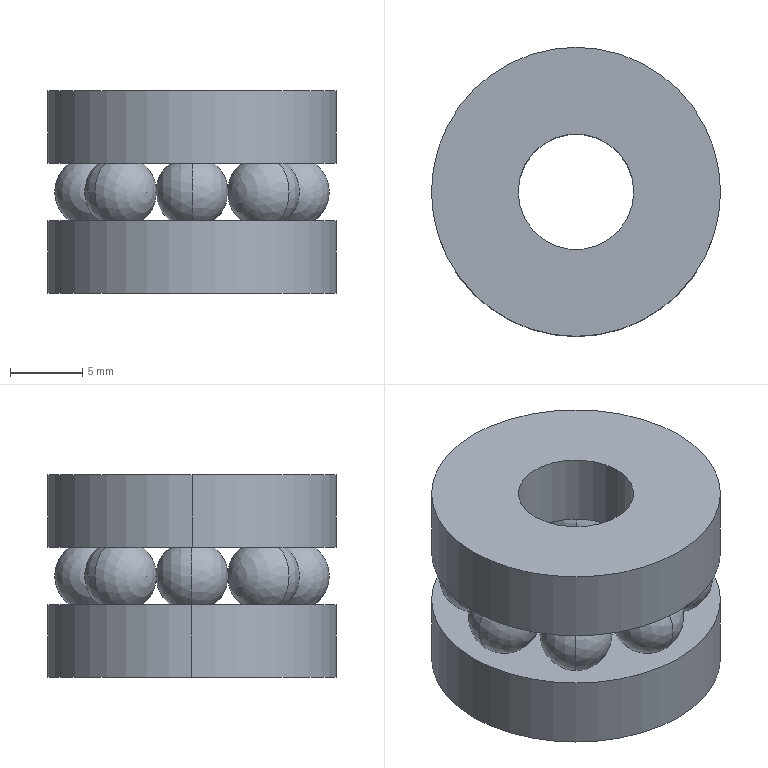Part | SolidWorks | features CirPattern 1, Extrusion 1, ICE 1, Revolution 1 | 1 solid | 28 faces | box 20 x 20 x 14 mm | volume 3133 mm3 | sphere 16 | cylinder 8 | plane 4 | commonest cylinder face diameters 8 x4 20 x4
STEP:
#1=CARTESIAN_POINT('',(-4.,0.,-4.));
#2=VERTEX_POINT('',#1);
#3=CARTESIAN_POINT('',(4.,0.,-4.));
#4=VERTEX_POINT('',#3);
#5=CARTESIAN_POINT('',(0.,0.,-4.));
#6=DIRECTION('',(0.,0.,1.));
#7=DIRECTION('',(1.,0.,0.));
#8=AXIS2_PLACEMENT_3D('',#5,#6,#7);
#9=CIRCLE('',#8,4.);
#10=EDGE_CURVE('',#2,#4,#9,.T.);
#11=ORIENTED_EDGE('',*,*,#10,.F.);
#12=CARTESIAN_POINT('',(-4.,0.,1.));
#13=VERTEX_POINT('',#12);
#14=CARTESIAN_POINT('',(-4.,0.,-4.));
#15=DIRECTION('',(0.,0.,1.));
#16=VECTOR('',#15,1000.);
#17=LINE('',#14,#16);
#18=EDGE_CURVE('',#2,#13,#17,.T.);
#19=ORIENTED_EDGE('',*,*,#18,.T.);
#20=CARTESIAN_POINT('',(4.,0.,1.));
#21=VERTEX_POINT('',#20);
#22=CARTESIAN_POINT('',(0.,0.,1.));
#23=DIRECTION('',(0.,0.,1.));
#24=DIRECTION('',(1.,0.,0.));
#25=AXIS2_PLACEMENT_3D('',#22,#23,#24);
#26=CIRCLE('',#25,4.);
#27=EDGE_CURVE('',#13,#21,#26,.T.);
#28=ORIENTED_EDGE('',*,*,#27,.T.);
#29=CARTESIAN_POINT('',(4.,0.,-4.));
#30=DIRECTION('',(0.,0.,1.));
#31=VECTOR('',#30,1000.);
#32=LINE('',#29,#31);
#33=EDGE_CURVE('',#4,#21,#32,.T.);
#34=ORIENTED_EDGE('',*,*,#33,.F.);
#35=EDGE_LOOP('',(#11,#19,#28,#34));
#36=FACE_OUTER_BOUND('',#35,.T.);
#37=CARTESIAN_POINT('',(0.,0.,-4.));
#38=DIRECTION('',(0.,0.,1.));
#39=DIRECTION('',(1.,0.,0.));
#40=AXIS2_PLACEMENT_3D('',#37,#38,#39);
#41=CYLINDRICAL_SURFACE('',#40,4.);
#42=ADVANCED_FACE('',(#36),#41,.F.);
#43=CARTESIAN_POINT('',(10.,0.,-4.));
#44=VERTEX_POINT('',#43);
#45=CARTESIAN_POINT('',(-10.,0.,-4.));
#46=VERTEX_POINT('',#45);
#47=CARTESIAN_POINT('',(0.,0.,-4.));
#48=DIRECTION('',(0.,0.,1.));
#49=DIRECTION('',(1.,0.,0.));
#50=AXIS2_PLACEMENT_3D('',#47,#48,#49);
#51=CIRCLE('',#50,10.);
#52=EDGE_CURVE('',#44,#46,#51,.T.);
#53=ORIENTED_EDGE('',*,*,#52,.T.);
#54=CARTESIAN_POINT('',(-10.,0.,1.));
#55=VERTEX_POINT('',#54);
#56=CARTESIAN_POINT('',(-10.,0.,-4.));
#57=DIRECTION('',(0.,0.,1.));
#58=VECTOR('',#57,1000.);
#59=LINE('',#56,#58);
#60=EDGE_CURVE('',#46,#55,#59,.T.);
#61=ORIENTED_EDGE('',*,*,#60,.T.);
#62=CARTESIAN_POINT('',(10.,0.,1.));
#63=VERTEX_POINT('',#62);
#64=CARTESIAN_POINT('',(0.,0.,1.));
#65=DIRECTION('',(0.,0.,1.));
#66=DIRECTION('',(1.,0.,0.));
#67=AXIS2_PLACEMENT_3D('',#64,#65,#66);
#68=CIRCLE('',#67,10.);
#69=EDGE_CURVE('',#63,#55,#68,.T.);
#70=ORIENTED_EDGE('',*,*,#69,.F.);
#71=CARTESIAN_POINT('',(10.,0.,-4.));
#72=DIRECTION('',(0.,0.,1.));
#73=VECTOR('',#72,1000.);
#74=LINE('',#71,#73);
#75=EDGE_CURVE('',#44,#63,#74,.T.);
#76=ORIENTED_EDGE('',*,*,#75,.F.);
#77=EDGE_LOOP('',(#53,#61,#70,#76));
#78=FACE_OUTER_BOUND('',#77,.T.);
#79=CARTESIAN_POINT('',(0.,0.,-4.));
#80=DIRECTION('',(0.,0.,1.));
#81=DIRECTION('',(1.,0.,0.));
#82=AXIS2_PLACEMENT_3D('',#79,#80,#81);
#83=CYLINDRICAL_SURFACE('',#82,10.);
#84=ADVANCED_FACE('',(#78),#83,.T.);
#85=CARTESIAN_POINT('',(-6.718,6.718,3.));
#86=VERTEX_POINT('',#85);
#87=CARTESIAN_POINT('',(-6.01,6.01,5.));
#88=VERTEX_POINT('',#87);
#89=CARTESIAN_POINT('',(-4.95,4.95,3.));
#90=DIRECTION('',(0.7071,0.7071,0.));
#91=DIRECTION('',(-0.7071,0.7071,0.));
#92=AXIS2_PLACEMENT_3D('',#89,#90,#91);
#93=CIRCLE('',#92,2.5);
#94=EDGE_CURVE('',#86,#88,#93,.T.);
#95=ORIENTED_EDGE('',*,*,#94,.F.);
#96=CARTESIAN_POINT('',(-6.01,6.01,1.));
#97=VERTEX_POINT('',#96);
#98=CARTESIAN_POINT('',(-4.95,4.95,3.));
#99=DIRECTION('',(-0.7071,-0.7071,0.));
#100=DIRECTION('',(0.7071,-0.7071,0.));
#101=AXIS2_PLACEMENT_3D('',#98,#99,#100);
#102=CIRCLE('',#101,2.5);
#103=EDGE_CURVE('',#86,#97,#102,.T.);
#104=ORIENTED_EDGE('',*,*,#103,.T.);
#105=CARTESIAN_POINT('',(-3.889,3.889,1.));
#106=VERTEX_POINT('',#105);
#107=CARTESIAN_POINT('',(-4.95,4.95,1.));
#108=DIRECTION('',(0.,0.,1.));
#109=DIRECTION('',(1.,0.,0.));
#110=AXIS2_PLACEMENT_3D('',#107,#108,#109);
#111=CIRCLE('',#110,1.5);
#112=EDGE_CURVE('',#97,#106,#111,.T.);
#113=ORIENTED_EDGE('',*,*,#112,.T.);
#114=CARTESIAN_POINT('',(-3.182,3.182,3.));
#115=VERTEX_POINT('',#114);
#116=CARTESIAN_POINT('',(-4.95,4.95,3.));
#117=DIRECTION('',(-0.7071,-0.7071,0.));
#118=DIRECTION('',(0.7071,-0.7071,0.));
#119=AXIS2_PLACEMENT_3D('',#116,#117,#118);
#120=CIRCLE('',#119,2.5);
#121=EDGE_CURVE('',#106,#115,#120,.T.);
#122=ORIENTED_EDGE('',*,*,#121,.T.);
#123=CARTESIAN_POINT('',(-3.889,3.889,5.));
#124=VERTEX_POINT('',#123);
#125=CARTESIAN_POINT('',(-4.95,4.95,3.));
#126=DIRECTION('',(0.7071,0.7071,0.));
#127=DIRECTION('',(-0.7071,0.7071,0.));
#128=AXIS2_PLACEMENT_3D('',#125,#126,#127);
#129=CIRCLE('',#128,2.5);
#130=EDGE_CURVE('',#124,#115,#129,.T.);
#131=ORIENTED_EDGE('',*,*,#130,.F.);
#132=CARTESIAN_POINT('',(-4.95,4.95,5.));
#133=DIRECTION('',(0.,0.,-1.));
#134=DIRECTION('',(1.,0.,0.));
#135=AXIS2_PLACEMENT_3D('',#132,#133,#134);
#136=CIRCLE('',#135,1.5);
#137=EDGE_CURVE('',#124,#88,#136,.T.);
#138=ORIENTED_EDGE('',*,*,#137,.T.);
#139=EDGE_LOOP('',(#95,#104,#113,#122,#131,#138));
#140=FACE_OUTER_BOUND('',#139,.T.);
#141=CARTESIAN_POINT('',(-4.95,4.95,3.));
#142=DIRECTION('',(-0.7071,-0.7071,0.));
#143=DIRECTION('',(0.,0.,1.));
#144=AXIS2_PLACEMENT_3D('',#141,#142,#143);
#145=SPHERICAL_SURFACE('',#144,2.5);
#146=ADVANCED_FACE('',(#140),#145,.T.);
#147=CARTESIAN_POINT('',(-9.5,0.,3.));
#148=VERTEX_POINT('',#147);
#149=CARTESIAN_POINT('',(-8.5,0.,5.));
#150=VERTEX_POINT('',#149);
#151=CARTESIAN_POINT('',(-7.,0.,3.));
#152=DIRECTION('',(0.,1.,0.));
#153=DIRECTION('',(-1.,0.,0.));
#154=AXIS2_PLACEMENT_3D('',#151,#152,#153);
#155=CIRCLE('',#154,2.5);
#156=EDGE_CURVE('',#148,#150,#155,.T.);
#157=ORIENTED_EDGE('',*,*,#156,.F.);
#158=CARTESIAN_POINT('',(-8.5,0.,1.));
#159=VERTEX_POINT('',#158);
#160=CARTESIAN_POINT('',(-7.,0.,3.));
#161=DIRECTION('',(0.,-1.,0.));
#162=DIRECTION('',(1.,0.,0.));
#163=AXIS2_PLACEMENT_3D('',#160,#161,#162);
#164=CIRCLE('',#163,2.5);
#165=EDGE_CURVE('',#148,#159,#164,.T.);
#166=ORIENTED_EDGE('',*,*,#165,.T.);
#167=CARTESIAN_POINT('',(-5.5,0.,1.));
#168=VERTEX_POINT('',#167);
#169=CARTESIAN_POINT('',(-7.,0.,1.));
#170=DIRECTION('',(0.,0.,1.));
#171=DIRECTION('',(1.,0.,0.));
#172=AXIS2_PLACEMENT_3D('',#169,#170,#171);
#173=CIRCLE('',#172,1.5);
#174=EDGE_CURVE('',#159,#168,#173,.T.);
#175=ORIENTED_EDGE('',*,*,#174,.T.);
#176=CARTESIAN_POINT('',(-4.5,0.,3.));
#177=VERTEX_POINT('',#176);
#178=CARTESIAN_POINT('',(-7.,0.,3.));
#179=DIRECTION('',(0.,-1.,0.));
#180=DIRECTION('',(1.,0.,0.));
#181=AXIS2_PLACEMENT_3D('',#178,#179,#180);
#182=CIRCLE('',#181,2.5);
#183=EDGE_CURVE('',#168,#177,#182,.T.);
#184=ORIENTED_EDGE('',*,*,#183,.T.);
#185=CARTESIAN_POINT('',(-5.5,0.,5.));
#186=VERTEX_POINT('',#185);
#187=CARTESIAN_POINT('',(-7.,0.,3.));
#188=DIRECTION('',(0.,1.,0.));
#189=DIRECTION('',(-1.,0.,0.));
#190=AXIS2_PLACEMENT_3D('',#187,#188,#189);
#191=CIRCLE('',#190,2.5);
#192=EDGE_CURVE('',#186,#177,#191,.T.);
#193=ORIENTED_EDGE('',*,*,#192,.F.);
#194=CARTESIAN_POINT('',(-7.,0.,5.));
#195=DIRECTION('',(0.,0.,-1.));
#196=DIRECTION('',(1.,0.,0.));
#197=AXIS2_PLACEMENT_3D('',#194,#195,#196);
#198=CIRCLE('',#197,1.5);
#199=EDGE_CURVE('',#186,#150,#198,.T.);
#200=ORIENTED_EDGE('',*,*,#199,.T.);
#201=EDGE_LOOP('',(#157,#166,#175,#184,#193,#200));
#202=FACE_OUTER_BOUND('',#201,.T.);
#203=CARTESIAN_POINT('',(-7.,0.,3.));
#204=DIRECTION('',(0.,-1.,0.));
#205=DIRECTION('',(0.,0.,1.));
#206=AXIS2_PLACEMENT_3D('',#203,#204,#205);
#207=SPHERICAL_SURFACE('',#206,2.5);
#208=ADVANCED_FACE('',(#202),#207,.T.);
#209=CARTESIAN_POINT('',(-6.718,-6.718,3.));
#210=VERTEX_POINT('',#209);
#211=CARTESIAN_POINT('',(-6.01,-6.01,5.));
#212=VERTEX_POINT('',#211);
#213=CARTESIAN_POINT('',(-4.95,-4.95,3.));
#214=DIRECTION('',(-0.7071,0.7071,0.));
#215=DIRECTION('',(-0.7071,-0.7071,0.));
#216=AXIS2_PLACEMENT_3D('',#213,#214,#215);
#217=CIRCLE('',#216,2.5);
#218=EDGE_CURVE('',#210,#212,#217,.T.);
#219=ORIENTED_EDGE('',*,*,#218,.F.);
#220=CARTESIAN_POINT('',(-6.01,-6.01,1.));
#221=VERTEX_POINT('',#220);
#222=CARTESIAN_POINT('',(-4.95,-4.95,3.));
#223=DIRECTION('',(0.7071,-0.7071,0.));
#224=DIRECTION('',(0.7071,0.7071,0.));
#225=AXIS2_PLACEMENT_3D('',#222,#223,#224);
#226=CIRCLE('',#225,2.5);
#227=EDGE_CURVE('',#210,#221,#226,.T.);
#228=ORIENTED_EDGE('',*,*,#227,.T.);
#229=CARTESIAN_POINT('',(-3.889,-3.889,1.));
#230=VERTEX_POINT('',#229);
#231=CARTESIAN_POINT('',(-4.95,-4.95,1.));
#232=DIRECTION('',(0.,0.,1.));
#233=DIRECTION('',(1.,0.,0.));
#234=AXIS2_PLACEMENT_3D('',#231,#232,#233);
#235=CIRCLE('',#234,1.5);
#236=EDGE_CURVE('',#221,#230,#235,.T.);
#237=ORIENTED_EDGE('',*,*,#236,.T.);
#238=CARTESIAN_POINT('',(-3.182,-3.182,3.));
#239=VERTEX_POINT('',#238);
#240=CARTESIAN_POINT('',(-4.95,-4.95,3.));
#241=DIRECTION('',(0.7071,-0.7071,0.));
#242=DIRECTION('',(0.7071,0.7071,0.));
#243=AXIS2_PLACEMENT_3D('',#240,#241,#242);
#244=CIRCLE('',#243,2.5);
#245=EDGE_CURVE('',#230,#239,#244,.T.);
#246=ORIENTED_EDGE('',*,*,#245,.T.);
#247=CARTESIAN_POINT('',(-3.889,-3.889,5.));
#248=VERTEX_POINT('',#247);
#249=CARTESIAN_POINT('',(-4.95,-4.95,3.));
#250=DIRECTION('',(-0.7071,0.7071,0.));
#251=DIRECTION('',(-0.7071,-0.7071,0.));
#252=AXIS2_PLACEMENT_3D('',#249,#250,#251);
#253=CIRCLE('',#252,2.5);
#254=EDGE_CURVE('',#248,#239,#253,.T.);
#255=ORIENTED_EDGE('',*,*,#254,.F.);
#256=CARTESIAN_POINT('',(-4.95,-4.95,5.));
#257=DIRECTION('',(0.,0.,-1.));
#258=DIRECTION('',(1.,0.,0.));
#259=AXIS2_PLACEMENT_3D('',#256,#257,#258);
#260=CIRCLE('',#259,1.5);
#261=EDGE_CURVE('',#248,#212,#260,.T.);
#262=ORIENTED_EDGE('',*,*,#261,.T.);
#263=EDGE_LOOP('',(#219,#228,#237,#246,#255,#262));
#264=FACE_OUTER_BOUND('',#263,.T.);
#265=CARTESIAN_POINT('',(-4.95,-4.95,3.));
#266=DIRECTION('',(0.7071,-0.7071,0.));
#267=DIRECTION('',(0.,0.,1.));
#268=AXIS2_PLACEMENT_3D('',#265,#266,#267);
#269=SPHERICAL_SURFACE('',#268,2.5);
#270=ADVANCED_FACE('',(#264),#269,.T.);
#271=CARTESIAN_POINT('',(0.,-9.5,3.));
#272=VERTEX_POINT('',#271);
#273=CARTESIAN_POINT('',(0.,-8.5,5.));
#274=VERTEX_POINT('',#273);
#275=CARTESIAN_POINT('',(0.,-7.,3.));
#276=DIRECTION('',(-1.,0.,0.));
#277=DIRECTION('',(0.,0.,1.));
#278=AXIS2_PLACEMENT_3D('',#275,#276,#277);
#279=CIRCLE('',#278,2.5);
#280=EDGE_CURVE('',#272,#274,#279,.T.);
#281=ORIENTED_EDGE('',*,*,#280,.F.);
#282=CARTESIAN_POINT('',(0.,-8.5,1.));
#283=VERTEX_POINT('',#282);
#284=CARTESIAN_POINT('',(0.,-7.,3.));
#285=DIRECTION('',(1.,0.,0.));
#286=DIRECTION('',(0.,0.,-1.));
#287=AXIS2_PLACEMENT_3D('',#284,#285,#286);
#288=CIRCLE('',#287,2.5);
#289=EDGE_CURVE('',#272,#283,#288,.T.);
#290=ORIENTED_EDGE('',*,*,#289,.T.);
#291=CARTESIAN_POINT('',(0.,-5.5,1.));
#292=VERTEX_POINT('',#291);
#293=CARTESIAN_POINT('',(0.,-7.,1.));
#294=DIRECTION('',(0.,0.,1.));
#295=DIRECTION('',(1.,0.,0.));
#296=AXIS2_PLACEMENT_3D('',#293,#294,#295);
#297=CIRCLE('',#296,1.5);
#298=EDGE_CURVE('',#283,#292,#297,.T.);
#299=ORIENTED_EDGE('',*,*,#298,.T.);
#300=CARTESIAN_POINT('',(0.,-4.5,3.));
#301=VERTEX_POINT('',#300);
#302=CARTESIAN_POINT('',(0.,-7.,3.));
#303=DIRECTION('',(1.,0.,0.));
#304=DIRECTION('',(0.,0.,-1.));
#305=AXIS2_PLACEMENT_3D('',#302,#303,#304);
#306=CIRCLE('',#305,2.5);
#307=EDGE_CURVE('',#292,#301,#306,.T.);
#308=ORIENTED_EDGE('',*,*,#307,.T.);
#309=CARTESIAN_POINT('',(0.,-5.5,5.));
#310=VERTEX_POINT('',#309);
#311=CARTESIAN_POINT('',(0.,-7.,3.));
#312=DIRECTION('',(-1.,0.,0.));
#313=DIRECTION('',(0.,0.,1.));
#314=AXIS2_PLACEMENT_3D('',#311,#312,#313);
#315=CIRCLE('',#314,2.5);
#316=EDGE_CURVE('',#310,#301,#315,.T.);
#317=ORIENTED_EDGE('',*,*,#316,.F.);
#318=CARTESIAN_POINT('',(0.,-7.,5.));
#319=DIRECTION('',(0.,0.,-1.));
#320=DIRECTION('',(1.,0.,0.));
#321=AXIS2_PLACEMENT_3D('',#318,#319,#320);
#322=CIRCLE('',#321,1.5);
#323=EDGE_CURVE('',#310,#274,#322,.T.);
#324=ORIENTED_EDGE('',*,*,#323,.T.);
#325=EDGE_LOOP('',(#281,#290,#299,#308,#317,#324));
#326=FACE_OUTER_BOUND('',#325,.T.);
#327=CARTESIAN_POINT('',(0.,-7.,3.));
#328=DIRECTION('',(1.,0.,0.));
#329=DIRECTION('',(0.,0.,1.));
#330=AXIS2_PLACEMENT_3D('',#327,#328,#329);
#331=SPHERICAL_SURFACE('',#330,2.5);
#332=ADVANCED_FACE('',(#326),#331,.T.);
#333=CARTESIAN_POINT('',(6.718,-6.718,3.));
#334=VERTEX_POINT('',#333);
#335=CARTESIAN_POINT('',(6.01,-6.01,5.));
#336=VERTEX_POINT('',#335);
#337=CARTESIAN_POINT('',(4.95,-4.95,3.));
#338=DIRECTION('',(-0.7071,-0.7071,0.));
#339=DIRECTION('',(0.7071,-0.7071,0.));
#340=AXIS2_PLACEMENT_3D('',#337,#338,#339);
#341=CIRCLE('',#340,2.5);
#342=EDGE_CURVE('',#334,#336,#341,.T.);
#343=ORIENTED_EDGE('',*,*,#342,.F.);
#344=CARTESIAN_POINT('',(6.01,-6.01,1.));
#345=VERTEX_POINT('',#344);
#346=CARTESIAN_POINT('',(4.95,-4.95,3.));
#347=DIRECTION('',(0.7071,0.7071,0.));
#348=DIRECTION('',(-0.7071,0.7071,0.));
#349=AXIS2_PLACEMENT_3D('',#346,#347,#348);
#350=CIRCLE('',#349,2.5);
#351=EDGE_CURVE('',#334,#345,#350,.T.);
#352=ORIENTED_EDGE('',*,*,#351,.T.);
#353=CARTESIAN_POINT('',(3.889,-3.889,1.));
#354=VERTEX_POINT('',#353);
#355=CARTESIAN_POINT('',(4.95,-4.95,1.));
#356=DIRECTION('',(0.,0.,1.));
#357=DIRECTION('',(1.,0.,0.));
#358=AXIS2_PLACEMENT_3D('',#355,#356,#357);
#359=CIRCLE('',#358,1.5);
#360=EDGE_CURVE('',#345,#354,#359,.T.);
#361=ORIENTED_EDGE('',*,*,#360,.T.);
#362=CARTESIAN_POINT('',(3.182,-3.182,3.));
#363=VERTEX_POINT('',#362);
#364=CARTESIAN_POINT('',(4.95,-4.95,3.));
#365=DIRECTION('',(0.7071,0.7071,0.));
#366=DIRECTION('',(-0.7071,0.7071,0.));
#367=AXIS2_PLACEMENT_3D('',#364,#365,#366);
#368=CIRCLE('',#367,2.5);
#369=EDGE_CURVE('',#354,#363,#368,.T.);
#370=ORIENTED_EDGE('',*,*,#369,.T.);
#371=CARTESIAN_POINT('',(3.889,-3.889,5.));
#372=VERTEX_POINT('',#371);
#373=CARTESIAN_POINT('',(4.95,-4.95,3.));
#374=DIRECTION('',(-0.7071,-0.7071,0.));
#375=DIRECTION('',(0.7071,-0.7071,0.));
#376=AXIS2_PLACEMENT_3D('',#373,#374,#375);
#377=CIRCLE('',#376,2.5);
#378=EDGE_CURVE('',#372,#363,#377,.T.);
#379=ORIENTED_EDGE('',*,*,#378,.F.);
#380=CARTESIAN_POINT('',(4.95,-4.95,5.));
#381=DIRECTION('',(0.,0.,-1.));
#382=DIRECTION('',(1.,0.,0.));
#383=AXIS2_PLACEMENT_3D('',#380,#381,#382);
#384=CIRCLE('',#383,1.5);
#385=EDGE_CURVE('',#372,#336,#384,.T.);
#386=ORIENTED_EDGE('',*,*,#385,.T.);
#387=EDGE_LOOP('',(#343,#352,#361,#370,#379,#386));
#388=FACE_OUTER_BOUND('',#387,.T.);
#389=CARTESIAN_POINT('',(4.95,-4.95,3.));
#390=DIRECTION('',(0.7071,0.7071,0.));
#391=DIRECTION('',(0.,0.,1.));
#392=AXIS2_PLACEMENT_3D('',#389,#390,#391);
#393=SPHERICAL_SURFACE('',#392,2.5);
#394=ADVANCED_FACE('',(#388),#393,.T.);
#395=CARTESIAN_POINT('',(9.5,0.,3.));
#396=VERTEX_POINT('',#395);
#397=CARTESIAN_POINT('',(8.5,0.,5.));
#398=VERTEX_POINT('',#397);
#399=CARTESIAN_POINT('',(7.,0.,3.));
#400=DIRECTION('',(0.,-1.,0.));
#401=DIRECTION('',(1.,0.,0.));
#402=AXIS2_PLACEMENT_3D('',#399,#400,#401);
#403=CIRCLE('',#402,2.5);
#404=EDGE_CURVE('',#396,#398,#403,.T.);
#405=ORIENTED_EDGE('',*,*,#404,.F.);
#406=CARTESIAN_POINT('',(8.5,0.,1.));
#407=VERTEX_POINT('',#406);
#408=CARTESIAN_POINT('',(7.,0.,3.));
#409=DIRECTION('',(0.,1.,0.));
#410=DIRECTION('',(-1.,0.,0.));
#411=AXIS2_PLACEMENT_3D('',#408,#409,#410);
#412=CIRCLE('',#411,2.5);
#413=EDGE_CURVE('',#396,#407,#412,.T.);
#414=ORIENTED_EDGE('',*,*,#413,.T.);
#415=CARTESIAN_POINT('',(5.5,0.,1.));
#416=VERTEX_POINT('',#415);
#417=CARTESIAN_POINT('',(7.,0.,1.));
#418=DIRECTION('',(0.,0.,1.));
#419=DIRECTION('',(1.,0.,0.));
#420=AXIS2_PLACEMENT_3D('',#417,#418,#419);
#421=CIRCLE('',#420,1.5);
#422=EDGE_CURVE('',#407,#416,#421,.T.);
#423=ORIENTED_EDGE('',*,*,#422,.T.);
#424=CARTESIAN_POINT('',(4.5,0.,3.));
#425=VERTEX_POINT('',#424);
#426=CARTESIAN_POINT('',(7.,0.,3.));
#427=DIRECTION('',(0.,1.,0.));
#428=DIRECTION('',(-1.,0.,0.));
#429=AXIS2_PLACEMENT_3D('',#426,#427,#428);
#430=CIRCLE('',#429,2.5);
#431=EDGE_CURVE('',#416,#425,#430,.T.);
#432=ORIENTED_EDGE('',*,*,#431,.T.);
#433=CARTESIAN_POINT('',(5.5,0.,5.));
#434=VERTEX_POINT('',#433);
#435=CARTESIAN_POINT('',(7.,0.,3.));
#436=DIRECTION('',(0.,-1.,0.));
#437=DIRECTION('',(1.,0.,0.));
#438=AXIS2_PLACEMENT_3D('',#435,#436,#437);
#439=CIRCLE('',#438,2.5);
#440=EDGE_CURVE('',#434,#425,#439,.T.);
#441=ORIENTED_EDGE('',*,*,#440,.F.);
#442=CARTESIAN_POINT('',(7.,0.,5.));
#443=DIRECTION('',(0.,0.,-1.));
#444=DIRECTION('',(1.,0.,0.));
#445=AXIS2_PLACEMENT_3D('',#442,#443,#444);
#446=CIRCLE('',#445,1.5);
#447=EDGE_CURVE('',#434,#398,#446,.T.);
#448=ORIENTED_EDGE('',*,*,#447,.T.);
#449=EDGE_LOOP('',(#405,#414,#423,#432,#441,#448));
#450=FACE_OUTER_BOUND('',#449,.T.);
#451=CARTESIAN_POINT('',(7.,0.,3.));
#452=DIRECTION('',(0.,1.,0.));
#453=DIRECTION('',(0.,0.,1.));
#454=AXIS2_PLACEMENT_3D('',#451,#452,#453);
#455=SPHERICAL_SURFACE('',#454,2.5);
#456=ADVANCED_FACE('',(#450),#455,.T.);
#457=CARTESIAN_POINT('',(6.718,6.718,3.));
#458=VERTEX_POINT('',#457);
#459=CARTESIAN_POINT('',(6.01,6.01,5.));
#460=VERTEX_POINT('',#459);
#461=CARTESIAN_POINT('',(4.95,4.95,3.));
#462=DIRECTION('',(0.7071,-0.7071,0.));
#463=DIRECTION('',(0.7071,0.7071,0.));
#464=AXIS2_PLACEMENT_3D('',#461,#462,#463);
#465=CIRCLE('',#464,2.5);
#466=EDGE_CURVE('',#458,#460,#465,.T.);
#467=ORIENTED_EDGE('',*,*,#466,.F.);
#468=CARTESIAN_POINT('',(6.01,6.01,1.));
#469=VERTEX_POINT('',#468);
#470=CARTESIAN_POINT('',(4.95,4.95,3.));
#471=DIRECTION('',(-0.7071,0.7071,0.));
#472=DIRECTION('',(-0.7071,-0.7071,0.));
#473=AXIS2_PLACEMENT_3D('',#470,#471,#472);
#474=CIRCLE('',#473,2.5);
#475=EDGE_CURVE('',#458,#469,#474,.T.);
#476=ORIENTED_EDGE('',*,*,#475,.T.);
#477=CARTESIAN_POINT('',(3.889,3.889,1.));
#478=VERTEX_POINT('',#477);
#479=CARTESIAN_POINT('',(4.95,4.95,1.));
#480=DIRECTION('',(0.,0.,1.));
#481=DIRECTION('',(1.,0.,0.));
#482=AXIS2_PLACEMENT_3D('',#479,#480,#481);
#483=CIRCLE('',#482,1.5);
#484=EDGE_CURVE('',#469,#478,#483,.T.);
#485=ORIENTED_EDGE('',*,*,#484,.T.);
#486=CARTESIAN_POINT('',(3.182,3.182,3.));
#487=VERTEX_POINT('',#486);
#488=CARTESIAN_POINT('',(4.95,4.95,3.));
#489=DIRECTION('',(-0.7071,0.7071,0.));
#490=DIRECTION('',(-0.7071,-0.7071,0.));
#491=AXIS2_PLACEMENT_3D('',#488,#489,#490);
#492=CIRCLE('',#491,2.5);
#493=EDGE_CURVE('',#478,#487,#492,.T.);
#494=ORIENTED_EDGE('',*,*,#493,.T.);
#495=CARTESIAN_POINT('',(3.889,3.889,5.));
#496=VERTEX_POINT('',#495);
#497=CARTESIAN_POINT('',(4.95,4.95,3.));
#498=DIRECTION('',(0.7071,-0.7071,0.));
#499=DIRECTION('',(0.7071,0.7071,0.));
#500=AXIS2_PLACEMENT_3D('',#497,#498,#499);
#501=CIRCLE('',#500,2.5);
#502=EDGE_CURVE('',#496,#487,#501,.T.);
#503=ORIENTED_EDGE('',*,*,#502,.F.);
#504=CARTESIAN_POINT('',(4.95,4.95,5.));
#505=DIRECTION('',(0.,0.,-1.));
#506=DIRECTION('',(1.,0.,0.));
#507=AXIS2_PLACEMENT_3D('',#504,#505,#506);
#508=CIRCLE('',#507,1.5);
#509=EDGE_CURVE('',#496,#460,#508,.T.);
#510=ORIENTED_EDGE('',*,*,#509,.T.);
#511=EDGE_LOOP('',(#467,#476,#485,#494,#503,#510));
#512=FACE_OUTER_BOUND('',#511,.T.);
#513=CARTESIAN_POINT('',(4.95,4.95,3.));
#514=DIRECTION('',(-0.7071,0.7071,0.));
#515=DIRECTION('',(0.,0.,1.));
#516=AXIS2_PLACEMENT_3D('',#513,#514,#515);
#517=SPHERICAL_SURFACE('',#516,2.5);
#518=ADVANCED_FACE('',(#512),#517,.T.);
#519=CARTESIAN_POINT('',(0.,9.5,3.));
#520=VERTEX_POINT('',#519);
#521=CARTESIAN_POINT('',(0.,8.5,5.));
#522=VERTEX_POINT('',#521);
#523=CARTESIAN_POINT('',(0.,7.,3.));
#524=DIRECTION('',(1.,0.,0.));
#525=DIRECTION('',(0.,0.,-1.));
#526=AXIS2_PLACEMENT_3D('',#523,#524,#525);
#527=CIRCLE('',#526,2.5);
#528=EDGE_CURVE('',#520,#522,#527,.T.);
#529=ORIENTED_EDGE('',*,*,#528,.F.);
#530=CARTESIAN_POINT('',(0.,8.5,1.));
#531=VERTEX_POINT('',#530);
#532=CARTESIAN_POINT('',(0.,7.,3.));
#533=DIRECTION('',(-1.,0.,0.));
#534=DIRECTION('',(0.,0.,1.));
#535=AXIS2_PLACEMENT_3D('',#532,#533,#534);
#536=CIRCLE('',#535,2.5);
#537=EDGE_CURVE('',#520,#531,#536,.T.);
#538=ORIENTED_EDGE('',*,*,#537,.T.);
#539=CARTESIAN_POINT('',(0.,5.5,1.));
#540=VERTEX_POINT('',#539);
#541=CARTESIAN_POINT('',(0.,7.,1.));
#542=DIRECTION('',(0.,0.,1.));
#543=DIRECTION('',(1.,0.,0.));
#544=AXIS2_PLACEMENT_3D('',#541,#542,#543);
#545=CIRCLE('',#544,1.5);
#546=EDGE_CURVE('',#531,#540,#545,.T.);
#547=ORIENTED_EDGE('',*,*,#546,.T.);
#548=CARTESIAN_POINT('',(0.,4.5,3.));
#549=VERTEX_POINT('',#548);
#550=CARTESIAN_POINT('',(0.,7.,3.));
#551=DIRECTION('',(-1.,0.,0.));
#552=DIRECTION('',(0.,0.,1.));
#553=AXIS2_PLACEMENT_3D('',#550,#551,#552);
#554=CIRCLE('',#553,2.5);
#555=EDGE_CURVE('',#540,#549,#554,.T.);
#556=ORIENTED_EDGE('',*,*,#555,.T.);
#557=CARTESIAN_POINT('',(0.,5.5,5.));
#558=VERTEX_POINT('',#557);
#559=CARTESIAN_POINT('',(0.,7.,3.));
#560=DIRECTION('',(1.,0.,0.));
#561=DIRECTION('',(0.,0.,-1.));
#562=AXIS2_PLACEMENT_3D('',#559,#560,#561);
#563=CIRCLE('',#562,2.5);
#564=EDGE_CURVE('',#558,#549,#563,.T.);
#565=ORIENTED_EDGE('',*,*,#564,.F.);
#566=CARTESIAN_POINT('',(0.,7.,5.));
#567=DIRECTION('',(0.,0.,-1.));
#568=DIRECTION('',(1.,0.,0.));
#569=AXIS2_PLACEMENT_3D('',#566,#567,#568);
#570=CIRCLE('',#569,1.5);
#571=EDGE_CURVE('',#558,#522,#570,.T.);
#572=ORIENTED_EDGE('',*,*,#571,.T.);
#573=EDGE_LOOP('',(#529,#538,#547,#556,#565,#572));
#574=FACE_OUTER_BOUND('',#573,.T.);
#575=CARTESIAN_POINT('',(0.,7.,3.));
#576=DIRECTION('',(-1.,0.,0.));
#577=DIRECTION('',(0.,0.,1.));
#578=AXIS2_PLACEMENT_3D('',#575,#576,#577);
#579=SPHERICAL_SURFACE('',#578,2.5);
#580=ADVANCED_FACE('',(#574),#579,.T.);
#581=CARTESIAN_POINT('',(-4.,0.,10.));
#582=VERTEX_POINT('',#581);
#583=CARTESIAN_POINT('',(4.,0.,10.));
#584=VERTEX_POINT('',#583);
#585=CARTESIAN_POINT('',(0.,0.,10.));
#586=DIRECTION('',(0.,0.,1.));
#587=DIRECTION('',(1.,0.,0.));
#588=AXIS2_PLACEMENT_3D('',#585,#586,#587);
#589=CIRCLE('',#588,4.);
#590=EDGE_CURVE('',#582,#584,#589,.T.);
#591=ORIENTED_EDGE('',*,*,#590,.T.);
#592=CARTESIAN_POINT('',(4.,0.,5.));
#593=VERTEX_POINT('',#592);
#594=CARTESIAN_POINT('',(4.,0.,10.));
#595=DIRECTION('',(0.,0.,-1.));
#596=VECTOR('',#595,1000.);
#597=LINE('',#594,#596);
#598=EDGE_CURVE('',#584,#593,#597,.T.);
#599=ORIENTED_EDGE('',*,*,#598,.T.);
#600=CARTESIAN_POINT('',(-4.,0.,5.));
#601=VERTEX_POINT('',#600);
#602=CARTESIAN_POINT('',(0.,0.,5.));
#603=DIRECTION('',(0.,0.,1.));
#604=DIRECTION('',(1.,0.,0.));
#605=AXIS2_PLACEMENT_3D('',#602,#603,#604);
#606=CIRCLE('',#605,4.);
#607=EDGE_CURVE('',#601,#593,#606,.T.);
#608=ORIENTED_EDGE('',*,*,#607,.F.);
#609=CARTESIAN_POINT('',(-4.,0.,10.));
#610=DIRECTION('',(0.,0.,-1.));
#611=VECTOR('',#610,1000.);
#612=LINE('',#609,#611);
#613=EDGE_CURVE('',#582,#601,#612,.T.);
#614=ORIENTED_EDGE('',*,*,#613,.F.);
#615=EDGE_LOOP('',(#591,#599,#608,#614));
#616=FACE_OUTER_BOUND('',#615,.T.);
#617=CARTESIAN_POINT('',(0.,0.,10.));
#618=DIRECTION('',(0.,0.,-1.));
#619=DIRECTION('',(-1.,0.,0.));
#620=AXIS2_PLACEMENT_3D('',#617,#618,#619);
#621=CYLINDRICAL_SURFACE('',#620,4.);
#622=ADVANCED_FACE('',(#616),#621,.F.);
#623=CARTESIAN_POINT('',(10.,0.,10.));
#624=VERTEX_POINT('',#623);
#625=CARTESIAN_POINT('',(-10.,0.,10.));
#626=VERTEX_POINT('',#625);
#627=CARTESIAN_POINT('',(0.,0.,10.));
#628=DIRECTION('',(0.,0.,1.));
#629=DIRECTION('',(1.,0.,0.));
#630=AXIS2_PLACEMENT_3D('',#627,#628,#629);
#631=CIRCLE('',#630,10.);
#632=EDGE_CURVE('',#624,#626,#631,.T.);
#633=ORIENTED_EDGE('',*,*,#632,.F.);
#634=CARTESIAN_POINT('',(10.,0.,5.));
#635=VERTEX_POINT('',#634);
#636=CARTESIAN_POINT('',(10.,0.,10.));
#637=DIRECTION('',(0.,0.,-1.));
#638=VECTOR('',#637,1000.);
#639=LINE('',#636,#638);
#640=EDGE_CURVE('',#624,#635,#639,.T.);
#641=ORIENTED_EDGE('',*,*,#640,.T.);
#642=CARTESIAN_POINT('',(-10.,0.,5.));
#643=VERTEX_POINT('',#642);
#644=CARTESIAN_POINT('',(0.,0.,5.));
#645=DIRECTION('',(0.,0.,1.));
#646=DIRECTION('',(1.,0.,0.));
#647=AXIS2_PLACEMENT_3D('',#644,#645,#646);
#648=CIRCLE('',#647,10.);
#649=EDGE_CURVE('',#635,#643,#648,.T.);
#650=ORIENTED_EDGE('',*,*,#649,.T.);
#651=CARTESIAN_POINT('',(-10.,0.,10.));
#652=DIRECTION('',(0.,0.,-1.));
#653=VECTOR('',#652,1000.);
#654=LINE('',#651,#653);
#655=EDGE_CURVE('',#626,#643,#654,.T.);
#656=ORIENTED_EDGE('',*,*,#655,.F.);
#657=EDGE_LOOP('',(#633,#641,#650,#656));
#658=FACE_OUTER_BOUND('',#657,.T.);
#659=CARTESIAN_POINT('',(0.,0.,10.));
#660=DIRECTION('',(0.,0.,-1.));
#661=DIRECTION('',(-1.,0.,0.));
#662=AXIS2_PLACEMENT_3D('',#659,#660,#661);
#663=CYLINDRICAL_SURFACE('',#662,10.);
#664=ADVANCED_FACE('',(#658),#663,.T.);
#665=CARTESIAN_POINT('',(0.,0.,10.));
#666=DIRECTION('',(0.,0.,1.));
#667=DIRECTION('',(1.,0.,0.));
#668=AXIS2_PLACEMENT_3D('',#665,#666,#667);
#669=CIRCLE('',#668,10.);
#670=EDGE_CURVE('',#626,#624,#669,.T.);
#671=ORIENTED_EDGE('',*,*,#670,.T.);
#672=ORIENTED_EDGE('',*,*,#632,.T.);
#673=EDGE_LOOP('',(#671,#672));
#674=FACE_OUTER_BOUND('',#673,.T.);
#675=ORIENTED_EDGE('',*,*,#590,.F.);
#676=CARTESIAN_POINT('',(0.,0.,10.));
#677=DIRECTION('',(0.,0.,1.));
#678=DIRECTION('',(1.,0.,0.));
#679=AXIS2_PLACEMENT_3D('',#676,#677,#678);
#680=CIRCLE('',#679,4.);
#681=EDGE_CURVE('',#584,#582,#680,.T.);
#682=ORIENTED_EDGE('',*,*,#681,.F.);
#683=EDGE_LOOP('',(#675,#682));
#684=FACE_BOUND('',#683,.T.);
#685=CARTESIAN_POINT('',(0.,0.,10.));
#686=DIRECTION('',(0.,0.,1.));
#687=DIRECTION('',(1.,0.,0.));
#688=AXIS2_PLACEMENT_3D('',#685,#686,#687);
#689=PLANE('',#688);
#690=ADVANCED_FACE('',(#674,#684),#689,.T.);
#691=ORIENTED_EDGE('',*,*,#137,.F.);
#692=CARTESIAN_POINT('',(-4.95,4.95,5.));
#693=DIRECTION('',(0.,0.,-1.));
#694=DIRECTION('',(1.,0.,0.));
#695=AXIS2_PLACEMENT_3D('',#692,#693,#694);
#696=CIRCLE('',#695,1.5);
#697=EDGE_CURVE('',#88,#124,#696,.T.);
#698=ORIENTED_EDGE('',*,*,#697,.F.);
#699=EDGE_LOOP('',(#691,#698));
#700=FACE_BOUND('',#699,.T.);
#701=ORIENTED_EDGE('',*,*,#199,.F.);
#702=CARTESIAN_POINT('',(-7.,0.,5.));
#703=DIRECTION('',(0.,0.,-1.));
#704=DIRECTION('',(1.,0.,0.));
#705=AXIS2_PLACEMENT_3D('',#702,#703,#704);
#706=CIRCLE('',#705,1.5);
#707=EDGE_CURVE('',#150,#186,#706,.T.);
#708=ORIENTED_EDGE('',*,*,#707,.F.);
#709=EDGE_LOOP('',(#701,#708));
#710=FACE_BOUND('',#709,.T.);
#711=CARTESIAN_POINT('',(-4.95,-4.95,5.));
#712=DIRECTION('',(0.,0.,-1.));
#713=DIRECTION('',(1.,0.,0.));
#714=AXIS2_PLACEMENT_3D('',#711,#712,#713);
#715=CIRCLE('',#714,1.5);
#716=EDGE_CURVE('',#212,#248,#715,.T.);
#717=ORIENTED_EDGE('',*,*,#716,.F.);
#718=ORIENTED_EDGE('',*,*,#261,.F.);
#719=EDGE_LOOP('',(#717,#718));
#720=FACE_BOUND('',#719,.T.);
#721=CARTESIAN_POINT('',(0.,-7.,5.));
#722=DIRECTION('',(0.,0.,-1.));
#723=DIRECTION('',(1.,0.,0.));
#724=AXIS2_PLACEMENT_3D('',#721,#722,#723);
#725=CIRCLE('',#724,1.5);
#726=EDGE_CURVE('',#274,#310,#725,.T.);
#727=ORIENTED_EDGE('',*,*,#726,.F.);
#728=ORIENTED_EDGE('',*,*,#323,.F.);
#729=EDGE_LOOP('',(#727,#728));
#730=FACE_BOUND('',#729,.T.);
#731=CARTESIAN_POINT('',(4.95,-4.95,5.));
#732=DIRECTION('',(0.,0.,-1.));
#733=DIRECTION('',(1.,0.,0.));
#734=AXIS2_PLACEMENT_3D('',#731,#732,#733);
#735=CIRCLE('',#734,1.5);
#736=EDGE_CURVE('',#336,#372,#735,.T.);
#737=ORIENTED_EDGE('',*,*,#736,.F.);
#738=ORIENTED_EDGE('',*,*,#385,.F.);
#739=EDGE_LOOP('',(#737,#738));
#740=FACE_BOUND('',#739,.T.);
#741=CARTESIAN_POINT('',(7.,0.,5.));
#742=DIRECTION('',(0.,0.,-1.));
#743=DIRECTION('',(1.,0.,0.));
#744=AXIS2_PLACEMENT_3D('',#741,#742,#743);
#745=CIRCLE('',#744,1.5);
#746=EDGE_CURVE('',#398,#434,#745,.T.);
#747=ORIENTED_EDGE('',*,*,#746,.F.);
#748=ORIENTED_EDGE('',*,*,#447,.F.);
#749=EDGE_LOOP('',(#747,#748));
#750=FACE_BOUND('',#749,.T.);
#751=ORIENTED_EDGE('',*,*,#509,.F.);
#752=CARTESIAN_POINT('',(4.95,4.95,5.));
#753=DIRECTION('',(0.,0.,-1.));
#754=DIRECTION('',(1.,0.,0.));
#755=AXIS2_PLACEMENT_3D('',#752,#753,#754);
#756=CIRCLE('',#755,1.5);
#757=EDGE_CURVE('',#460,#496,#756,.T.);
#758=ORIENTED_EDGE('',*,*,#757,.F.);
#759=EDGE_LOOP('',(#751,#758));
#760=FACE_BOUND('',#759,.T.);
#761=ORIENTED_EDGE('',*,*,#571,.F.);
#762=CARTESIAN_POINT('',(0.,7.,5.));
#763=DIRECTION('',(0.,0.,-1.));
#764=DIRECTION('',(1.,0.,0.));
#765=AXIS2_PLACEMENT_3D('',#762,#763,#764);
#766=CIRCLE('',#765,1.5);
#767=EDGE_CURVE('',#522,#558,#766,.T.);
#768=ORIENTED_EDGE('',*,*,#767,.F.);
#769=EDGE_LOOP('',(#761,#768));
#770=FACE_BOUND('',#769,.T.);
#771=CARTESIAN_POINT('',(0.,0.,5.));
#772=DIRECTION('',(0.,0.,1.));
#773=DIRECTION('',(1.,0.,0.));
#774=AXIS2_PLACEMENT_3D('',#771,#772,#773);
#775=CIRCLE('',#774,10.);
#776=EDGE_CURVE('',#643,#635,#775,.T.);
#777=ORIENTED_EDGE('',*,*,#776,.F.);
#778=ORIENTED_EDGE('',*,*,#649,.F.);
#779=EDGE_LOOP('',(#777,#778));
#780=FACE_OUTER_BOUND('',#779,.T.);
#781=ORIENTED_EDGE('',*,*,#607,.T.);
#782=CARTESIAN_POINT('',(0.,0.,5.));
#783=DIRECTION('',(0.,0.,1.));
#784=DIRECTION('',(1.,0.,0.));
#785=AXIS2_PLACEMENT_3D('',#782,#783,#784);
#786=CIRCLE('',#785,4.);
#787=EDGE_CURVE('',#593,#601,#786,.T.);
#788=ORIENTED_EDGE('',*,*,#787,.T.);
#789=EDGE_LOOP('',(#781,#788));
#790=FACE_BOUND('',#789,.T.);
#791=CARTESIAN_POINT('',(0.,0.,5.));
#792=DIRECTION('',(0.,0.,1.));
#793=DIRECTION('',(1.,0.,0.));
#794=AXIS2_PLACEMENT_3D('',#791,#792,#793);
#795=PLANE('',#794);
#796=ADVANCED_FACE('',(#700,#710,#720,#730,#740,#750,#760,#770,#780,#790),#795,.F.);
#797=ORIENTED_EDGE('',*,*,#640,.F.);
#798=ORIENTED_EDGE('',*,*,#670,.F.);
#799=ORIENTED_EDGE('',*,*,#655,.T.);
#800=ORIENTED_EDGE('',*,*,#776,.T.);
#801=EDGE_LOOP('',(#797,#798,#799,#800));
#802=FACE_OUTER_BOUND('',#801,.T.);
#803=CARTESIAN_POINT('',(0.,0.,10.));
#804=DIRECTION('',(0.,0.,-1.));
#805=DIRECTION('',(-1.,0.,0.));
#806=AXIS2_PLACEMENT_3D('',#803,#804,#805);
#807=CYLINDRICAL_SURFACE('',#806,10.);
#808=ADVANCED_FACE('',(#802),#807,.T.);
#809=ORIENTED_EDGE('',*,*,#598,.F.);
#810=ORIENTED_EDGE('',*,*,#681,.T.);
#811=ORIENTED_EDGE('',*,*,#613,.T.);
#812=ORIENTED_EDGE('',*,*,#787,.F.);
#813=EDGE_LOOP('',(#809,#810,#811,#812));
#814=FACE_OUTER_BOUND('',#813,.T.);
#815=CARTESIAN_POINT('',(0.,0.,10.));
#816=DIRECTION('',(0.,0.,-1.));
#817=DIRECTION('',(-1.,0.,0.));
#818=AXIS2_PLACEMENT_3D('',#815,#816,#817);
#819=CYLINDRICAL_SURFACE('',#818,4.);
#820=ADVANCED_FACE('',(#814),#819,.F.);
#821=ORIENTED_EDGE('',*,*,#537,.F.);
#822=ORIENTED_EDGE('',*,*,#528,.T.);
#823=ORIENTED_EDGE('',*,*,#767,.T.);
#824=ORIENTED_EDGE('',*,*,#564,.T.);
#825=ORIENTED_EDGE('',*,*,#555,.F.);
#826=CARTESIAN_POINT('',(0.,7.,1.));
#827=DIRECTION('',(0.,0.,1.));
#828=DIRECTION('',(1.,0.,0.));
#829=AXIS2_PLACEMENT_3D('',#826,#827,#828);
#830=CIRCLE('',#829,1.5);
#831=EDGE_CURVE('',#540,#531,#830,.T.);
#832=ORIENTED_EDGE('',*,*,#831,.T.);
#833=EDGE_LOOP('',(#821,#822,#823,#824,#825,#832));
#834=FACE_OUTER_BOUND('',#833,.T.);
#835=CARTESIAN_POINT('',(0.,7.,3.));
#836=DIRECTION('',(-1.,0.,0.));
#837=DIRECTION('',(0.,0.,1.));
#838=AXIS2_PLACEMENT_3D('',#835,#836,#837);
#839=SPHERICAL_SURFACE('',#838,2.5);
#840=ADVANCED_FACE('',(#834),#839,.T.);
#841=ORIENTED_EDGE('',*,*,#475,.F.);
#842=ORIENTED_EDGE('',*,*,#466,.T.);
#843=ORIENTED_EDGE('',*,*,#757,.T.);
#844=ORIENTED_EDGE('',*,*,#502,.T.);
#845=ORIENTED_EDGE('',*,*,#493,.F.);
#846=CARTESIAN_POINT('',(4.95,4.95,1.));
#847=DIRECTION('',(0.,0.,1.));
#848=DIRECTION('',(1.,0.,0.));
#849=AXIS2_PLACEMENT_3D('',#846,#847,#848);
#850=CIRCLE('',#849,1.5);
#851=EDGE_CURVE('',#478,#469,#850,.T.);
#852=ORIENTED_EDGE('',*,*,#851,.T.);
#853=EDGE_LOOP('',(#841,#842,#843,#844,#845,#852));
#854=FACE_OUTER_BOUND('',#853,.T.);
#855=CARTESIAN_POINT('',(4.95,4.95,3.));
#856=DIRECTION('',(-0.7071,0.7071,0.));
#857=DIRECTION('',(0.,0.,1.));
#858=AXIS2_PLACEMENT_3D('',#855,#856,#857);
#859=SPHERICAL_SURFACE('',#858,2.5);
#860=ADVANCED_FACE('',(#854),#859,.T.);
#861=ORIENTED_EDGE('',*,*,#413,.F.);
#862=ORIENTED_EDGE('',*,*,#404,.T.);
#863=ORIENTED_EDGE('',*,*,#746,.T.);
#864=ORIENTED_EDGE('',*,*,#440,.T.);
#865=ORIENTED_EDGE('',*,*,#431,.F.);
#866=CARTESIAN_POINT('',(7.,0.,1.));
#867=DIRECTION('',(0.,0.,1.));
#868=DIRECTION('',(1.,0.,0.));
#869=AXIS2_PLACEMENT_3D('',#866,#867,#868);
#870=CIRCLE('',#869,1.5);
#871=EDGE_CURVE('',#416,#407,#870,.T.);
#872=ORIENTED_EDGE('',*,*,#871,.T.);
#873=EDGE_LOOP('',(#861,#862,#863,#864,#865,#872));
#874=FACE_OUTER_BOUND('',#873,.T.);
#875=CARTESIAN_POINT('',(7.,0.,3.));
#876=DIRECTION('',(0.,1.,0.));
#877=DIRECTION('',(0.,0.,1.));
#878=AXIS2_PLACEMENT_3D('',#875,#876,#877);
#879=SPHERICAL_SURFACE('',#878,2.5);
#880=ADVANCED_FACE('',(#874),#879,.T.);
#881=ORIENTED_EDGE('',*,*,#351,.F.);
#882=ORIENTED_EDGE('',*,*,#342,.T.);
#883=ORIENTED_EDGE('',*,*,#736,.T.);
#884=ORIENTED_EDGE('',*,*,#378,.T.);
#885=ORIENTED_EDGE('',*,*,#369,.F.);
#886=CARTESIAN_POINT('',(4.95,-4.95,1.));
#887=DIRECTION('',(0.,0.,1.));
#888=DIRECTION('',(1.,0.,0.));
#889=AXIS2_PLACEMENT_3D('',#886,#887,#888);
#890=CIRCLE('',#889,1.5);
#891=EDGE_CURVE('',#354,#345,#890,.T.);
#892=ORIENTED_EDGE('',*,*,#891,.T.);
#893=EDGE_LOOP('',(#881,#882,#883,#884,#885,#892));
#894=FACE_OUTER_BOUND('',#893,.T.);
#895=CARTESIAN_POINT('',(4.95,-4.95,3.));
#896=DIRECTION('',(0.7071,0.7071,0.));
#897=DIRECTION('',(0.,0.,1.));
#898=AXIS2_PLACEMENT_3D('',#895,#896,#897);
#899=SPHERICAL_SURFACE('',#898,2.5);
#900=ADVANCED_FACE('',(#894),#899,.T.);
#901=ORIENTED_EDGE('',*,*,#289,.F.);
#902=ORIENTED_EDGE('',*,*,#280,.T.);
#903=ORIENTED_EDGE('',*,*,#726,.T.);
#904=ORIENTED_EDGE('',*,*,#316,.T.);
#905=ORIENTED_EDGE('',*,*,#307,.F.);
#906=CARTESIAN_POINT('',(0.,-7.,1.));
#907=DIRECTION('',(0.,0.,1.));
#908=DIRECTION('',(1.,0.,0.));
#909=AXIS2_PLACEMENT_3D('',#906,#907,#908);
#910=CIRCLE('',#909,1.5);
#911=EDGE_CURVE('',#292,#283,#910,.T.);
#912=ORIENTED_EDGE('',*,*,#911,.T.);
#913=EDGE_LOOP('',(#901,#902,#903,#904,#905,#912));
#914=FACE_OUTER_BOUND('',#913,.T.);
#915=CARTESIAN_POINT('',(0.,-7.,3.));
#916=DIRECTION('',(1.,0.,0.));
#917=DIRECTION('',(0.,0.,1.));
#918=AXIS2_PLACEMENT_3D('',#915,#916,#917);
#919=SPHERICAL_SURFACE('',#918,2.5);
#920=ADVANCED_FACE('',(#914),#919,.T.);
#921=ORIENTED_EDGE('',*,*,#227,.F.);
#922=ORIENTED_EDGE('',*,*,#218,.T.);
#923=ORIENTED_EDGE('',*,*,#716,.T.);
#924=ORIENTED_EDGE('',*,*,#254,.T.);
#925=ORIENTED_EDGE('',*,*,#245,.F.);
#926=CARTESIAN_POINT('',(-4.95,-4.95,1.));
#927=DIRECTION('',(0.,0.,1.));
#928=DIRECTION('',(1.,0.,0.));
#929=AXIS2_PLACEMENT_3D('',#926,#927,#928);
#930=CIRCLE('',#929,1.5);
#931=EDGE_CURVE('',#230,#221,#930,.T.);
#932=ORIENTED_EDGE('',*,*,#931,.T.);
#933=EDGE_LOOP('',(#921,#922,#923,#924,#925,#932));
#934=FACE_OUTER_BOUND('',#933,.T.);
#935=CARTESIAN_POINT('',(-4.95,-4.95,3.));
#936=DIRECTION('',(0.7071,-0.7071,0.));
#937=DIRECTION('',(0.,0.,1.));
#938=AXIS2_PLACEMENT_3D('',#935,#936,#937);
#939=SPHERICAL_SURFACE('',#938,2.5);
#940=ADVANCED_FACE('',(#934),#939,.T.);
#941=ORIENTED_EDGE('',*,*,#165,.F.);
#942=ORIENTED_EDGE('',*,*,#156,.T.);
#943=ORIENTED_EDGE('',*,*,#707,.T.);
#944=ORIENTED_EDGE('',*,*,#192,.T.);
#945=ORIENTED_EDGE('',*,*,#183,.F.);
#946=CARTESIAN_POINT('',(-7.,0.,1.));
#947=DIRECTION('',(0.,0.,1.));
#948=DIRECTION('',(1.,0.,0.));
#949=AXIS2_PLACEMENT_3D('',#946,#947,#948);
#950=CIRCLE('',#949,1.5);
#951=EDGE_CURVE('',#168,#159,#950,.T.);
#952=ORIENTED_EDGE('',*,*,#951,.T.);
#953=EDGE_LOOP('',(#941,#942,#943,#944,#945,#952));
#954=FACE_OUTER_BOUND('',#953,.T.);
#955=CARTESIAN_POINT('',(-7.,0.,3.));
#956=DIRECTION('',(0.,-1.,0.));
#957=DIRECTION('',(0.,0.,1.));
#958=AXIS2_PLACEMENT_3D('',#955,#956,#957);
#959=SPHERICAL_SURFACE('',#958,2.5);
#960=ADVANCED_FACE('',(#954),#959,.T.);
#961=ORIENTED_EDGE('',*,*,#103,.F.);
#962=ORIENTED_EDGE('',*,*,#94,.T.);
#963=ORIENTED_EDGE('',*,*,#697,.T.);
#964=ORIENTED_EDGE('',*,*,#130,.T.);
#965=ORIENTED_EDGE('',*,*,#121,.F.);
#966=CARTESIAN_POINT('',(-4.95,4.95,1.));
#967=DIRECTION('',(0.,0.,1.));
#968=DIRECTION('',(1.,0.,0.));
#969=AXIS2_PLACEMENT_3D('',#966,#967,#968);
#970=CIRCLE('',#969,1.5);
#971=EDGE_CURVE('',#106,#97,#970,.T.);
#972=ORIENTED_EDGE('',*,*,#971,.T.);
#973=EDGE_LOOP('',(#961,#962,#963,#964,#965,#972));
#974=FACE_OUTER_BOUND('',#973,.T.);
#975=CARTESIAN_POINT('',(-4.95,4.95,3.));
#976=DIRECTION('',(-0.7071,-0.7071,0.));
#977=DIRECTION('',(0.,0.,1.));
#978=AXIS2_PLACEMENT_3D('',#975,#976,#977);
#979=SPHERICAL_SURFACE('',#978,2.5);
#980=ADVANCED_FACE('',(#974),#979,.T.);
#981=ORIENTED_EDGE('',*,*,#60,.F.);
#982=CARTESIAN_POINT('',(0.,0.,-4.));
#983=DIRECTION('',(0.,0.,1.));
#984=DIRECTION('',(1.,0.,0.));
#985=AXIS2_PLACEMENT_3D('',#982,#983,#984);
#986=CIRCLE('',#985,10.);
#987=EDGE_CURVE('',#46,#44,#986,.T.);
#988=ORIENTED_EDGE('',*,*,#987,.T.);
#989=ORIENTED_EDGE('',*,*,#75,.T.);
#990=CARTESIAN_POINT('',(0.,0.,1.));
#991=DIRECTION('',(0.,0.,1.));
#992=DIRECTION('',(1.,0.,0.));
#993=AXIS2_PLACEMENT_3D('',#990,#991,#992);
#994=CIRCLE('',#993,10.);
#995=EDGE_CURVE('',#55,#63,#994,.T.);
#996=ORIENTED_EDGE('',*,*,#995,.F.);
#997=EDGE_LOOP('',(#981,#988,#989,#996));
#998=FACE_OUTER_BOUND('',#997,.T.);
#999=CARTESIAN_POINT('',(0.,0.,-4.));
#1000=DIRECTION('',(0.,0.,1.));
#1001=DIRECTION('',(1.,0.,0.));
#1002=AXIS2_PLACEMENT_3D('',#999,#1000,#1001);
#1003=CYLINDRICAL_SURFACE('',#1002,10.);
#1004=ADVANCED_FACE('',(#998),#1003,.T.);
#1005=CARTESIAN_POINT('',(0.,0.,-4.));
#1006=DIRECTION('',(0.,0.,1.));
#1007=DIRECTION('',(1.,0.,0.));
#1008=AXIS2_PLACEMENT_3D('',#1005,#1006,#1007);
#1009=CIRCLE('',#1008,4.);
#1010=EDGE_CURVE('',#4,#2,#1009,.T.);
#1011=ORIENTED_EDGE('',*,*,#1010,.T.);
#1012=ORIENTED_EDGE('',*,*,#10,.T.);
#1013=EDGE_LOOP('',(#1011,#1012));
#1014=FACE_BOUND('',#1013,.T.);
#1015=ORIENTED_EDGE('',*,*,#52,.F.);
#1016=ORIENTED_EDGE('',*,*,#987,.F.);
#1017=EDGE_LOOP('',(#1015,#1016));
#1018=FACE_OUTER_BOUND('',#1017,.T.);
#1019=CARTESIAN_POINT('',(0.,0.,-4.));
#1020=DIRECTION('',(0.,0.,1.));
#1021=DIRECTION('',(1.,0.,0.));
#1022=AXIS2_PLACEMENT_3D('',#1019,#1020,#1021);
#1023=PLANE('',#1022);
#1024=ADVANCED_FACE('',(#1014,#1018),#1023,.F.);
#1025=ORIENTED_EDGE('',*,*,#546,.F.);
#1026=ORIENTED_EDGE('',*,*,#831,.F.);
#1027=EDGE_LOOP('',(#1025,#1026));
#1028=FACE_BOUND('',#1027,.T.);
#1029=ORIENTED_EDGE('',*,*,#484,.F.);
#1030=ORIENTED_EDGE('',*,*,#851,.F.);
#1031=EDGE_LOOP('',(#1029,#1030));
#1032=FACE_BOUND('',#1031,.T.);
#1033=ORIENTED_EDGE('',*,*,#422,.F.);
#1034=ORIENTED_EDGE('',*,*,#871,.F.);
#1035=EDGE_LOOP('',(#1033,#1034));
#1036=FACE_BOUND('',#1035,.T.);
#1037=ORIENTED_EDGE('',*,*,#891,.F.);
#1038=ORIENTED_EDGE('',*,*,#360,.F.);
#1039=EDGE_LOOP('',(#1037,#1038));
#1040=FACE_BOUND('',#1039,.T.);
#1041=ORIENTED_EDGE('',*,*,#911,.F.);
#1042=ORIENTED_EDGE('',*,*,#298,.F.);
#1043=EDGE_LOOP('',(#1041,#1042));
#1044=FACE_BOUND('',#1043,.T.);
#1045=ORIENTED_EDGE('',*,*,#931,.F.);
#1046=ORIENTED_EDGE('',*,*,#236,.F.);
#1047=EDGE_LOOP('',(#1045,#1046));
#1048=FACE_BOUND('',#1047,.T.);
#1049=ORIENTED_EDGE('',*,*,#951,.F.);
#1050=ORIENTED_EDGE('',*,*,#174,.F.);
#1051=EDGE_LOOP('',(#1049,#1050));
#1052=FACE_BOUND('',#1051,.T.);
#1053=ORIENTED_EDGE('',*,*,#112,.F.);
#1054=ORIENTED_EDGE('',*,*,#971,.F.);
#1055=EDGE_LOOP('',(#1053,#1054));
#1056=FACE_BOUND('',#1055,.T.);
#1057=CARTESIAN_POINT('',(0.,0.,1.));
#1058=DIRECTION('',(0.,0.,1.));
#1059=DIRECTION('',(1.,0.,0.));
#1060=AXIS2_PLACEMENT_3D('',#1057,#1058,#1059);
#1061=CIRCLE('',#1060,4.);
#1062=EDGE_CURVE('',#21,#13,#1061,.T.);
#1063=ORIENTED_EDGE('',*,*,#1062,.F.);
#1064=ORIENTED_EDGE('',*,*,#27,.F.);
#1065=EDGE_LOOP('',(#1063,#1064));
#1066=FACE_BOUND('',#1065,.T.);
#1067=ORIENTED_EDGE('',*,*,#69,.T.);
#1068=ORIENTED_EDGE('',*,*,#995,.T.);
#1069=EDGE_LOOP('',(#1067,#1068));
#1070=FACE_OUTER_BOUND('',#1069,.T.);
#1071=CARTESIAN_POINT('',(0.,0.,1.));
#1072=DIRECTION('',(0.,0.,1.));
#1073=DIRECTION('',(1.,0.,0.));
#1074=AXIS2_PLACEMENT_3D('',#1071,#1072,#1073);
#1075=PLANE('',#1074);
#1076=ADVANCED_FACE('',(#1028,#1032,#1036,#1040,#1044,#1048,#1052,#1056,#1066,#1070),#1075,.T.);
#1077=ORIENTED_EDGE('',*,*,#18,.F.);
#1078=ORIENTED_EDGE('',*,*,#1010,.F.);
#1079=ORIENTED_EDGE('',*,*,#33,.T.);
#1080=ORIENTED_EDGE('',*,*,#1062,.T.);
#1081=EDGE_LOOP('',(#1077,#1078,#1079,#1080));
#1082=FACE_OUTER_BOUND('',#1081,.T.);
#1083=CARTESIAN_POINT('',(0.,0.,-4.));
#1084=DIRECTION('',(0.,0.,1.));
#1085=DIRECTION('',(1.,0.,0.));
#1086=AXIS2_PLACEMENT_3D('',#1083,#1084,#1085);
#1087=CYLINDRICAL_SURFACE('',#1086,4.);
#1088=ADVANCED_FACE('',(#1082),#1087,.F.);
#1089=CLOSED_SHELL('',(#42,#84,#146,#208,#270,#332,#394,#456,#518,#580,#622,#664,#690,#796,#808,#820,#840,#860,#880,#900,#920,#940,#960,#980,#1004,#1024,#1076,#1088));
#1090=MANIFOLD_SOLID_BREP('',#1089);
#1091=CARTESIAN_POINT('',(0.,0.,0.));
#1092=DIRECTION('',(0.,0.,1.));
#1093=DIRECTION('',(1.,0.,0.));
#1094=AXIS2_PLACEMENT_3D('',#1091,#1092,#1093);
#1095=(LENGTH_UNIT()NAMED_UNIT(*)SI_UNIT(.MILLI.,.METRE.));
#1096=UNCERTAINTY_MEASURE_WITH_UNIT(LENGTH_MEASURE(0.00001),#1095,'','');
#1097=(NAMED_UNIT(*)PLANE_ANGLE_UNIT()SI_UNIT($,.RADIAN.));
#1098=(NAMED_UNIT(*)SI_UNIT($,.STERADIAN.)SOLID_ANGLE_UNIT());
#1099=(GEOMETRIC_REPRESENTATION_CONTEXT(3)GLOBAL_UNCERTAINTY_ASSIGNED_CONTEXT((#1096))GLOBAL_UNIT_ASSIGNED_CONTEXT((#1095,#1097,#1098))REPRESENTATION_CONTEXT('',''));
#1100=ADVANCED_BREP_SHAPE_REPRESENTATION('',(#1090,#1094),#1099);